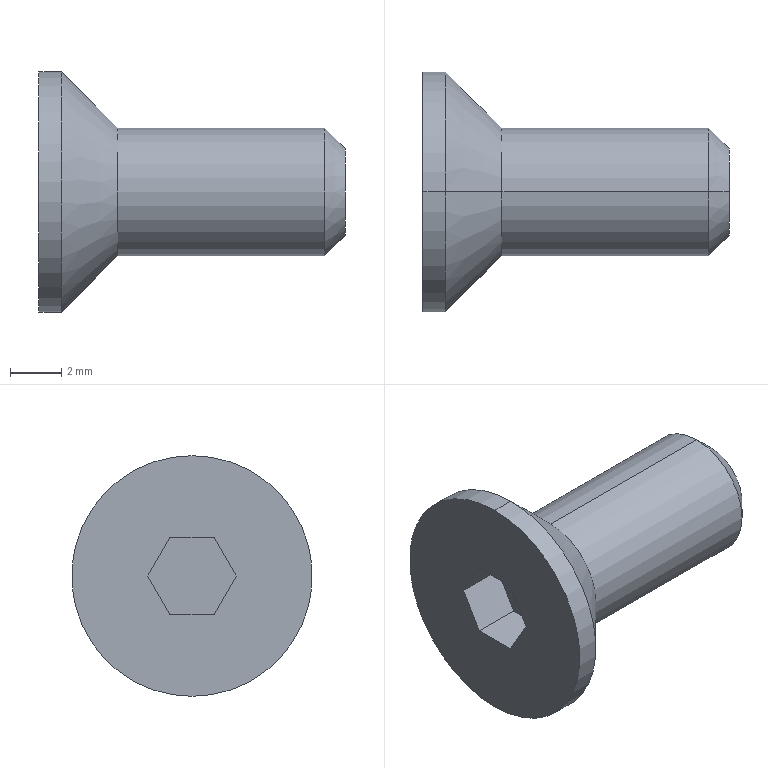Part | STEP file | Flat-head hex socket screw Dongming full thread M5-12 A2-70-1 | 1 solid | 17 faces | box 12 x 9.43 x 9.43 mm | volume 310.666 mm3 | plane 9 | cylinder 4 | cone 4 | commonest cylinder face diameters 5 x2 9.43 x2
STEP:
#1=CARTESIAN_POINT('',(0.885,0.,4.715));
#2=VERTEX_POINT('',#1);
#3=CARTESIAN_POINT('',(0.885,0.,-4.715));
#4=VERTEX_POINT('',#3);
#5=CARTESIAN_POINT('',(0.885,0.,0.));
#6=DIRECTION('',(-1.,0.,0.));
#7=DIRECTION('',(0.,0.,1.));
#8=AXIS2_PLACEMENT_3D('',#5,#6,#7);
#9=CIRCLE('',#8,4.715);
#10=EDGE_CURVE('',#2,#4,#9,.T.);
#11=ORIENTED_EDGE('',*,*,#10,.T.);
#12=CARTESIAN_POINT('',(0.,0.,-4.715));
#13=VERTEX_POINT('',#12);
#14=CARTESIAN_POINT('',(0.,0.,-4.715));
#15=DIRECTION('',(-1.,0.,0.));
#16=VECTOR('',#15,1000.);
#17=LINE('',#14,#16);
#18=EDGE_CURVE('',#4,#13,#17,.T.);
#19=ORIENTED_EDGE('',*,*,#18,.T.);
#20=CARTESIAN_POINT('',(0.,0.,4.715));
#21=VERTEX_POINT('',#20);
#22=CARTESIAN_POINT('',(0.,0.,0.));
#23=DIRECTION('',(-1.,0.,0.));
#24=DIRECTION('',(0.,0.,1.));
#25=AXIS2_PLACEMENT_3D('',#22,#23,#24);
#26=CIRCLE('',#25,4.715);
#27=EDGE_CURVE('',#21,#13,#26,.T.);
#28=ORIENTED_EDGE('',*,*,#27,.F.);
#29=CARTESIAN_POINT('',(0.,0.,4.715));
#30=DIRECTION('',(-1.,0.,0.));
#31=VECTOR('',#30,1000.);
#32=LINE('',#29,#31);
#33=EDGE_CURVE('',#2,#21,#32,.T.);
#34=ORIENTED_EDGE('',*,*,#33,.F.);
#35=EDGE_LOOP('',(#11,#19,#28,#34));
#36=FACE_OUTER_BOUND('',#35,.T.);
#37=CARTESIAN_POINT('',(0.,0.,0.));
#38=DIRECTION('',(-1.,0.,0.));
#39=DIRECTION('',(0.,0.,1.));
#40=AXIS2_PLACEMENT_3D('',#37,#38,#39);
#41=CYLINDRICAL_SURFACE('',#40,4.715);
#42=ADVANCED_FACE('',(#36),#41,.T.);
#43=CARTESIAN_POINT('',(3.1,0.,2.5));
#44=VERTEX_POINT('',#43);
#45=CARTESIAN_POINT('',(3.1,0.,-2.5));
#46=VERTEX_POINT('',#45);
#47=CARTESIAN_POINT('',(3.1,0.,0.));
#48=DIRECTION('',(-1.,0.,0.));
#49=DIRECTION('',(0.,0.,1.));
#50=AXIS2_PLACEMENT_3D('',#47,#48,#49);
#51=CIRCLE('',#50,2.5);
#52=EDGE_CURVE('',#44,#46,#51,.T.);
#53=ORIENTED_EDGE('',*,*,#52,.T.);
#54=CARTESIAN_POINT('',(3.1,0.,-2.5));
#55=DIRECTION('',(-0.7071,0.,-0.7071));
#56=VECTOR('',#55,1000.);
#57=LINE('',#54,#56);
#58=EDGE_CURVE('',#46,#4,#57,.T.);
#59=ORIENTED_EDGE('',*,*,#58,.T.);
#60=ORIENTED_EDGE('',*,*,#10,.F.);
#61=CARTESIAN_POINT('',(3.1,0.,2.5));
#62=DIRECTION('',(-0.7071,0.,0.7071));
#63=VECTOR('',#62,1000.);
#64=LINE('',#61,#63);
#65=EDGE_CURVE('',#44,#2,#64,.T.);
#66=ORIENTED_EDGE('',*,*,#65,.F.);
#67=EDGE_LOOP('',(#53,#59,#60,#66));
#68=FACE_OUTER_BOUND('',#67,.T.);
#69=CARTESIAN_POINT('',(3.1,0.,0.));
#70=DIRECTION('',(-1.,0.,0.));
#71=DIRECTION('',(0.,0.,1.));
#72=AXIS2_PLACEMENT_3D('',#69,#70,#71);
#73=CONICAL_SURFACE('',#72,2.5,0.7854);
#74=ADVANCED_FACE('',(#68),#73,.T.);
#75=CARTESIAN_POINT('',(11.2,0.,2.5));
#76=VERTEX_POINT('',#75);
#77=CARTESIAN_POINT('',(11.2,0.,-2.5));
#78=VERTEX_POINT('',#77);
#79=CARTESIAN_POINT('',(11.2,0.,0.));
#80=DIRECTION('',(-1.,0.,0.));
#81=DIRECTION('',(0.,0.,1.));
#82=AXIS2_PLACEMENT_3D('',#79,#80,#81);
#83=CIRCLE('',#82,2.5);
#84=EDGE_CURVE('',#76,#78,#83,.T.);
#85=ORIENTED_EDGE('',*,*,#84,.T.);
#86=CARTESIAN_POINT('',(0.,0.,-2.5));
#87=DIRECTION('',(-1.,0.,0.));
#88=VECTOR('',#87,1000.);
#89=LINE('',#86,#88);
#90=EDGE_CURVE('',#78,#46,#89,.T.);
#91=ORIENTED_EDGE('',*,*,#90,.T.);
#92=ORIENTED_EDGE('',*,*,#52,.F.);
#93=CARTESIAN_POINT('',(0.,0.,2.5));
#94=DIRECTION('',(-1.,0.,0.));
#95=VECTOR('',#94,1000.);
#96=LINE('',#93,#95);
#97=EDGE_CURVE('',#76,#44,#96,.T.);
#98=ORIENTED_EDGE('',*,*,#97,.F.);
#99=EDGE_LOOP('',(#85,#91,#92,#98));
#100=FACE_OUTER_BOUND('',#99,.T.);
#101=CARTESIAN_POINT('',(0.,0.,0.));
#102=DIRECTION('',(-1.,0.,0.));
#103=DIRECTION('',(0.,0.,1.));
#104=AXIS2_PLACEMENT_3D('',#101,#102,#103);
#105=CYLINDRICAL_SURFACE('',#104,2.5);
#106=ADVANCED_FACE('',(#100),#105,.T.);
#107=CARTESIAN_POINT('',(12.,0.,1.7));
#108=VERTEX_POINT('',#107);
#109=CARTESIAN_POINT('',(12.,0.,-1.7));
#110=VERTEX_POINT('',#109);
#111=CARTESIAN_POINT('',(12.,0.,0.));
#112=DIRECTION('',(-1.,0.,0.));
#113=DIRECTION('',(0.,0.,1.));
#114=AXIS2_PLACEMENT_3D('',#111,#112,#113);
#115=CIRCLE('',#114,1.7);
#116=EDGE_CURVE('',#108,#110,#115,.T.);
#117=ORIENTED_EDGE('',*,*,#116,.T.);
#118=CARTESIAN_POINT('',(12.,0.,-1.7));
#119=DIRECTION('',(-0.7071,0.,-0.7071));
#120=VECTOR('',#119,1000.);
#121=LINE('',#118,#120);
#122=EDGE_CURVE('',#110,#78,#121,.T.);
#123=ORIENTED_EDGE('',*,*,#122,.T.);
#124=ORIENTED_EDGE('',*,*,#84,.F.);
#125=CARTESIAN_POINT('',(12.,0.,1.7));
#126=DIRECTION('',(-0.7071,0.,0.7071));
#127=VECTOR('',#126,1000.);
#128=LINE('',#125,#127);
#129=EDGE_CURVE('',#108,#76,#128,.T.);
#130=ORIENTED_EDGE('',*,*,#129,.F.);
#131=EDGE_LOOP('',(#117,#123,#124,#130));
#132=FACE_OUTER_BOUND('',#131,.T.);
#133=CARTESIAN_POINT('',(12.,0.,0.));
#134=DIRECTION('',(-1.,0.,0.));
#135=DIRECTION('',(0.,0.,1.));
#136=AXIS2_PLACEMENT_3D('',#133,#134,#135);
#137=CONICAL_SURFACE('',#136,1.7,0.7854);
#138=ADVANCED_FACE('',(#132),#137,.T.);
#139=ORIENTED_EDGE('',*,*,#116,.F.);
#140=CARTESIAN_POINT('',(12.,0.,0.));
#141=DIRECTION('',(-1.,0.,0.));
#142=DIRECTION('',(0.,0.,1.));
#143=AXIS2_PLACEMENT_3D('',#140,#141,#142);
#144=CIRCLE('',#143,1.7);
#145=EDGE_CURVE('',#110,#108,#144,.T.);
#146=ORIENTED_EDGE('',*,*,#145,.F.);
#147=EDGE_LOOP('',(#139,#146));
#148=FACE_OUTER_BOUND('',#147,.T.);
#149=CARTESIAN_POINT('',(12.,0.,0.));
#150=DIRECTION('',(-1.,0.,0.));
#151=DIRECTION('',(0.,0.,1.));
#152=AXIS2_PLACEMENT_3D('',#149,#150,#151);
#153=PLANE('',#152);
#154=ADVANCED_FACE('',(#148),#153,.F.);
#155=ORIENTED_EDGE('',*,*,#122,.F.);
#156=ORIENTED_EDGE('',*,*,#145,.T.);
#157=ORIENTED_EDGE('',*,*,#129,.T.);
#158=CARTESIAN_POINT('',(11.2,0.,0.));
#159=DIRECTION('',(-1.,0.,0.));
#160=DIRECTION('',(0.,0.,1.));
#161=AXIS2_PLACEMENT_3D('',#158,#159,#160);
#162=CIRCLE('',#161,2.5);
#163=EDGE_CURVE('',#78,#76,#162,.T.);
#164=ORIENTED_EDGE('',*,*,#163,.F.);
#165=EDGE_LOOP('',(#155,#156,#157,#164));
#166=FACE_OUTER_BOUND('',#165,.T.);
#167=CARTESIAN_POINT('',(12.,0.,0.));
#168=DIRECTION('',(-1.,0.,0.));
#169=DIRECTION('',(0.,0.,1.));
#170=AXIS2_PLACEMENT_3D('',#167,#168,#169);
#171=CONICAL_SURFACE('',#170,1.7,0.7854);
#172=ADVANCED_FACE('',(#166),#171,.T.);
#173=ORIENTED_EDGE('',*,*,#90,.F.);
#174=ORIENTED_EDGE('',*,*,#163,.T.);
#175=ORIENTED_EDGE('',*,*,#97,.T.);
#176=CARTESIAN_POINT('',(3.1,0.,0.));
#177=DIRECTION('',(-1.,0.,0.));
#178=DIRECTION('',(0.,0.,1.));
#179=AXIS2_PLACEMENT_3D('',#176,#177,#178);
#180=CIRCLE('',#179,2.5);
#181=EDGE_CURVE('',#46,#44,#180,.T.);
#182=ORIENTED_EDGE('',*,*,#181,.F.);
#183=EDGE_LOOP('',(#173,#174,#175,#182));
#184=FACE_OUTER_BOUND('',#183,.T.);
#185=CARTESIAN_POINT('',(0.,0.,0.));
#186=DIRECTION('',(-1.,0.,0.));
#187=DIRECTION('',(0.,0.,1.));
#188=AXIS2_PLACEMENT_3D('',#185,#186,#187);
#189=CYLINDRICAL_SURFACE('',#188,2.5);
#190=ADVANCED_FACE('',(#184),#189,.T.);
#191=ORIENTED_EDGE('',*,*,#58,.F.);
#192=ORIENTED_EDGE('',*,*,#181,.T.);
#193=ORIENTED_EDGE('',*,*,#65,.T.);
#194=CARTESIAN_POINT('',(0.885,0.,0.));
#195=DIRECTION('',(-1.,0.,0.));
#196=DIRECTION('',(0.,0.,1.));
#197=AXIS2_PLACEMENT_3D('',#194,#195,#196);
#198=CIRCLE('',#197,4.715);
#199=EDGE_CURVE('',#4,#2,#198,.T.);
#200=ORIENTED_EDGE('',*,*,#199,.F.);
#201=EDGE_LOOP('',(#191,#192,#193,#200));
#202=FACE_OUTER_BOUND('',#201,.T.);
#203=CARTESIAN_POINT('',(3.1,0.,0.));
#204=DIRECTION('',(-1.,0.,0.));
#205=DIRECTION('',(0.,0.,1.));
#206=AXIS2_PLACEMENT_3D('',#203,#204,#205);
#207=CONICAL_SURFACE('',#206,2.5,0.7854);
#208=ADVANCED_FACE('',(#202),#207,.T.);
#209=ORIENTED_EDGE('',*,*,#18,.F.);
#210=ORIENTED_EDGE('',*,*,#199,.T.);
#211=ORIENTED_EDGE('',*,*,#33,.T.);
#212=CARTESIAN_POINT('',(0.,0.,0.));
#213=DIRECTION('',(-1.,0.,0.));
#214=DIRECTION('',(0.,0.,1.));
#215=AXIS2_PLACEMENT_3D('',#212,#213,#214);
#216=CIRCLE('',#215,4.715);
#217=EDGE_CURVE('',#13,#21,#216,.T.);
#218=ORIENTED_EDGE('',*,*,#217,.F.);
#219=EDGE_LOOP('',(#209,#210,#211,#218));
#220=FACE_OUTER_BOUND('',#219,.T.);
#221=CARTESIAN_POINT('',(0.,0.,0.));
#222=DIRECTION('',(-1.,0.,0.));
#223=DIRECTION('',(0.,0.,1.));
#224=AXIS2_PLACEMENT_3D('',#221,#222,#223);
#225=CYLINDRICAL_SURFACE('',#224,4.715);
#226=ADVANCED_FACE('',(#220),#225,.T.);
#227=CARTESIAN_POINT('',(0.,1.732,0.));
#228=VERTEX_POINT('',#227);
#229=CARTESIAN_POINT('',(0.,0.866,-1.5));
#230=VERTEX_POINT('',#229);
#231=CARTESIAN_POINT('',(0.,1.732,0.));
#232=DIRECTION('',(0.,-0.5,-0.866));
#233=VECTOR('',#232,1000.);
#234=LINE('',#231,#233);
#235=EDGE_CURVE('',#228,#230,#234,.T.);
#236=ORIENTED_EDGE('',*,*,#235,.F.);
#237=CARTESIAN_POINT('',(0.,0.866,1.5));
#238=VERTEX_POINT('',#237);
#239=CARTESIAN_POINT('',(0.,0.866,1.5));
#240=DIRECTION('',(0.,0.5,-0.866));
#241=VECTOR('',#240,1000.);
#242=LINE('',#239,#241);
#243=EDGE_CURVE('',#238,#228,#242,.T.);
#244=ORIENTED_EDGE('',*,*,#243,.F.);
#245=CARTESIAN_POINT('',(0.,-0.866,1.5));
#246=VERTEX_POINT('',#245);
#247=CARTESIAN_POINT('',(0.,-0.866,1.5));
#248=DIRECTION('',(0.,1.,0.));
#249=VECTOR('',#248,1000.);
#250=LINE('',#247,#249);
#251=EDGE_CURVE('',#246,#238,#250,.T.);
#252=ORIENTED_EDGE('',*,*,#251,.F.);
#253=CARTESIAN_POINT('',(0.,-1.732,0.));
#254=VERTEX_POINT('',#253);
#255=CARTESIAN_POINT('',(0.,-1.732,0.));
#256=DIRECTION('',(0.,0.5,0.866));
#257=VECTOR('',#256,1000.);
#258=LINE('',#255,#257);
#259=EDGE_CURVE('',#254,#246,#258,.T.);
#260=ORIENTED_EDGE('',*,*,#259,.F.);
#261=CARTESIAN_POINT('',(0.,-0.866,-1.5));
#262=VERTEX_POINT('',#261);
#263=CARTESIAN_POINT('',(0.,-0.866,-1.5));
#264=DIRECTION('',(0.,-0.5,0.866));
#265=VECTOR('',#264,1000.);
#266=LINE('',#263,#265);
#267=EDGE_CURVE('',#262,#254,#266,.T.);
#268=ORIENTED_EDGE('',*,*,#267,.F.);
#269=CARTESIAN_POINT('',(0.,0.866,-1.5));
#270=DIRECTION('',(0.,-1.,0.));
#271=VECTOR('',#270,1000.);
#272=LINE('',#269,#271);
#273=EDGE_CURVE('',#230,#262,#272,.T.);
#274=ORIENTED_EDGE('',*,*,#273,.F.);
#275=EDGE_LOOP('',(#236,#244,#252,#260,#268,#274));
#276=FACE_BOUND('',#275,.T.);
#277=ORIENTED_EDGE('',*,*,#27,.T.);
#278=ORIENTED_EDGE('',*,*,#217,.T.);
#279=EDGE_LOOP('',(#277,#278));
#280=FACE_OUTER_BOUND('',#279,.T.);
#281=CARTESIAN_POINT('',(0.,4.715,0.));
#282=DIRECTION('',(1.,0.,0.));
#283=DIRECTION('',(0.,0.,-1.));
#284=AXIS2_PLACEMENT_3D('',#281,#282,#283);
#285=PLANE('',#284);
#286=ADVANCED_FACE('',(#276,#280),#285,.F.);
#287=ORIENTED_EDGE('',*,*,#243,.T.);
#288=CARTESIAN_POINT('',(1.9,1.732,0.));
#289=VERTEX_POINT('',#288);
#290=CARTESIAN_POINT('',(1.9,1.732,0.));
#291=DIRECTION('',(-1.,0.,0.));
#292=VECTOR('',#291,1000.);
#293=LINE('',#290,#292);
#294=EDGE_CURVE('',#289,#228,#293,.T.);
#295=ORIENTED_EDGE('',*,*,#294,.F.);
#296=CARTESIAN_POINT('',(1.9,0.866,1.5));
#297=VERTEX_POINT('',#296);
#298=CARTESIAN_POINT('',(1.9,0.866,1.5));
#299=DIRECTION('',(0.,0.5,-0.866));
#300=VECTOR('',#299,1000.);
#301=LINE('',#298,#300);
#302=EDGE_CURVE('',#297,#289,#301,.T.);
#303=ORIENTED_EDGE('',*,*,#302,.F.);
#304=CARTESIAN_POINT('',(1.9,0.866,1.5));
#305=DIRECTION('',(-1.,0.,0.));
#306=VECTOR('',#305,1000.);
#307=LINE('',#304,#306);
#308=EDGE_CURVE('',#297,#238,#307,.T.);
#309=ORIENTED_EDGE('',*,*,#308,.T.);
#310=EDGE_LOOP('',(#287,#295,#303,#309));
#311=FACE_OUTER_BOUND('',#310,.T.);
#312=CARTESIAN_POINT('',(1.9,0.866,1.5));
#313=DIRECTION('',(0.,0.866,0.5));
#314=DIRECTION('',(0.,-0.5,0.866));
#315=AXIS2_PLACEMENT_3D('',#312,#313,#314);
#316=PLANE('',#315);
#317=ADVANCED_FACE('',(#311),#316,.F.);
#318=ORIENTED_EDGE('',*,*,#251,.T.);
#319=ORIENTED_EDGE('',*,*,#308,.F.);
#320=CARTESIAN_POINT('',(1.9,-0.866,1.5));
#321=VERTEX_POINT('',#320);
#322=CARTESIAN_POINT('',(1.9,-0.866,1.5));
#323=DIRECTION('',(0.,1.,0.));
#324=VECTOR('',#323,1000.);
#325=LINE('',#322,#324);
#326=EDGE_CURVE('',#321,#297,#325,.T.);
#327=ORIENTED_EDGE('',*,*,#326,.F.);
#328=CARTESIAN_POINT('',(1.9,-0.866,1.5));
#329=DIRECTION('',(-1.,0.,0.));
#330=VECTOR('',#329,1000.);
#331=LINE('',#328,#330);
#332=EDGE_CURVE('',#321,#246,#331,.T.);
#333=ORIENTED_EDGE('',*,*,#332,.T.);
#334=EDGE_LOOP('',(#318,#319,#327,#333));
#335=FACE_OUTER_BOUND('',#334,.T.);
#336=CARTESIAN_POINT('',(1.9,-0.866,1.5));
#337=DIRECTION('',(0.,0.,1.));
#338=DIRECTION('',(1.,0.,0.));
#339=AXIS2_PLACEMENT_3D('',#336,#337,#338);
#340=PLANE('',#339);
#341=ADVANCED_FACE('',(#335),#340,.F.);
#342=ORIENTED_EDGE('',*,*,#259,.T.);
#343=ORIENTED_EDGE('',*,*,#332,.F.);
#344=CARTESIAN_POINT('',(1.9,-1.732,0.));
#345=VERTEX_POINT('',#344);
#346=CARTESIAN_POINT('',(1.9,-1.732,0.));
#347=DIRECTION('',(0.,0.5,0.866));
#348=VECTOR('',#347,1000.);
#349=LINE('',#346,#348);
#350=EDGE_CURVE('',#345,#321,#349,.T.);
#351=ORIENTED_EDGE('',*,*,#350,.F.);
#352=CARTESIAN_POINT('',(1.9,-1.732,0.));
#353=DIRECTION('',(-1.,0.,0.));
#354=VECTOR('',#353,1000.);
#355=LINE('',#352,#354);
#356=EDGE_CURVE('',#345,#254,#355,.T.);
#357=ORIENTED_EDGE('',*,*,#356,.T.);
#358=EDGE_LOOP('',(#342,#343,#351,#357));
#359=FACE_OUTER_BOUND('',#358,.T.);
#360=CARTESIAN_POINT('',(1.9,-1.732,0.));
#361=DIRECTION('',(0.,-0.866,0.5));
#362=DIRECTION('',(0.,-0.5,-0.866));
#363=AXIS2_PLACEMENT_3D('',#360,#361,#362);
#364=PLANE('',#363);
#365=ADVANCED_FACE('',(#359),#364,.F.);
#366=ORIENTED_EDGE('',*,*,#267,.T.);
#367=ORIENTED_EDGE('',*,*,#356,.F.);
#368=CARTESIAN_POINT('',(1.9,-0.866,-1.5));
#369=VERTEX_POINT('',#368);
#370=CARTESIAN_POINT('',(1.9,-0.866,-1.5));
#371=DIRECTION('',(0.,-0.5,0.866));
#372=VECTOR('',#371,1000.);
#373=LINE('',#370,#372);
#374=EDGE_CURVE('',#369,#345,#373,.T.);
#375=ORIENTED_EDGE('',*,*,#374,.F.);
#376=CARTESIAN_POINT('',(1.9,-0.866,-1.5));
#377=DIRECTION('',(-1.,0.,0.));
#378=VECTOR('',#377,1000.);
#379=LINE('',#376,#378);
#380=EDGE_CURVE('',#369,#262,#379,.T.);
#381=ORIENTED_EDGE('',*,*,#380,.T.);
#382=EDGE_LOOP('',(#366,#367,#375,#381));
#383=FACE_OUTER_BOUND('',#382,.T.);
#384=CARTESIAN_POINT('',(1.9,-0.866,-1.5));
#385=DIRECTION('',(0.,-0.866,-0.5));
#386=DIRECTION('',(0.,0.5,-0.866));
#387=AXIS2_PLACEMENT_3D('',#384,#385,#386);
#388=PLANE('',#387);
#389=ADVANCED_FACE('',(#383),#388,.F.);
#390=ORIENTED_EDGE('',*,*,#273,.T.);
#391=ORIENTED_EDGE('',*,*,#380,.F.);
#392=CARTESIAN_POINT('',(1.9,0.866,-1.5));
#393=VERTEX_POINT('',#392);
#394=CARTESIAN_POINT('',(1.9,0.866,-1.5));
#395=DIRECTION('',(0.,-1.,0.));
#396=VECTOR('',#395,1000.);
#397=LINE('',#394,#396);
#398=EDGE_CURVE('',#393,#369,#397,.T.);
#399=ORIENTED_EDGE('',*,*,#398,.F.);
#400=CARTESIAN_POINT('',(1.9,0.866,-1.5));
#401=DIRECTION('',(-1.,0.,0.));
#402=VECTOR('',#401,1000.);
#403=LINE('',#400,#402);
#404=EDGE_CURVE('',#393,#230,#403,.T.);
#405=ORIENTED_EDGE('',*,*,#404,.T.);
#406=EDGE_LOOP('',(#390,#391,#399,#405));
#407=FACE_OUTER_BOUND('',#406,.T.);
#408=CARTESIAN_POINT('',(1.9,0.866,-1.5));
#409=DIRECTION('',(0.,0.,-1.));
#410=DIRECTION('',(0.,1.,0.));
#411=AXIS2_PLACEMENT_3D('',#408,#409,#410);
#412=PLANE('',#411);
#413=ADVANCED_FACE('',(#407),#412,.F.);
#414=ORIENTED_EDGE('',*,*,#235,.T.);
#415=ORIENTED_EDGE('',*,*,#404,.F.);
#416=CARTESIAN_POINT('',(1.9,1.732,0.));
#417=DIRECTION('',(0.,-0.5,-0.866));
#418=VECTOR('',#417,1000.);
#419=LINE('',#416,#418);
#420=EDGE_CURVE('',#289,#393,#419,.T.);
#421=ORIENTED_EDGE('',*,*,#420,.F.);
#422=ORIENTED_EDGE('',*,*,#294,.T.);
#423=EDGE_LOOP('',(#414,#415,#421,#422));
#424=FACE_OUTER_BOUND('',#423,.T.);
#425=CARTESIAN_POINT('',(1.9,1.732,0.));
#426=DIRECTION('',(0.,0.866,-0.5));
#427=DIRECTION('',(0.,0.5,0.866));
#428=AXIS2_PLACEMENT_3D('',#425,#426,#427);
#429=PLANE('',#428);
#430=ADVANCED_FACE('',(#424),#429,.F.);
#431=ORIENTED_EDGE('',*,*,#302,.T.);
#432=ORIENTED_EDGE('',*,*,#420,.T.);
#433=ORIENTED_EDGE('',*,*,#398,.T.);
#434=ORIENTED_EDGE('',*,*,#374,.T.);
#435=ORIENTED_EDGE('',*,*,#350,.T.);
#436=ORIENTED_EDGE('',*,*,#326,.T.);
#437=EDGE_LOOP('',(#431,#432,#433,#434,#435,#436));
#438=FACE_OUTER_BOUND('',#437,.T.);
#439=CARTESIAN_POINT('',(1.9,0.,0.));
#440=DIRECTION('',(-1.,0.,0.));
#441=DIRECTION('',(0.,0.,1.));
#442=AXIS2_PLACEMENT_3D('',#439,#440,#441);
#443=PLANE('',#442);
#444=ADVANCED_FACE('',(#438),#443,.T.);
#445=CLOSED_SHELL('',(#42,#74,#106,#138,#154,#172,#190,#208,#226,#286,#317,#341,#365,#389,#413,#430,#444));
#446=MANIFOLD_SOLID_BREP('',#445);
#447=CARTESIAN_POINT('',(0.,0.,0.));
#448=DIRECTION('',(0.,0.,1.));
#449=DIRECTION('',(1.,0.,0.));
#450=AXIS2_PLACEMENT_3D('',#447,#448,#449);
#451=(LENGTH_UNIT()NAMED_UNIT(*)SI_UNIT(.MILLI.,.METRE.));
#452=UNCERTAINTY_MEASURE_WITH_UNIT(LENGTH_MEASURE(0.00001),#451,'','');
#453=(NAMED_UNIT(*)PLANE_ANGLE_UNIT()SI_UNIT($,.RADIAN.));
#454=(NAMED_UNIT(*)SI_UNIT($,.STERADIAN.)SOLID_ANGLE_UNIT());
#455=(GEOMETRIC_REPRESENTATION_CONTEXT(3)GLOBAL_UNCERTAINTY_ASSIGNED_CONTEXT((#452))GLOBAL_UNIT_ASSIGNED_CONTEXT((#451,#453,#454))REPRESENTATION_CONTEXT('',''));
#456=ADVANCED_BREP_SHAPE_REPRESENTATION('',(#446,#450),#455);